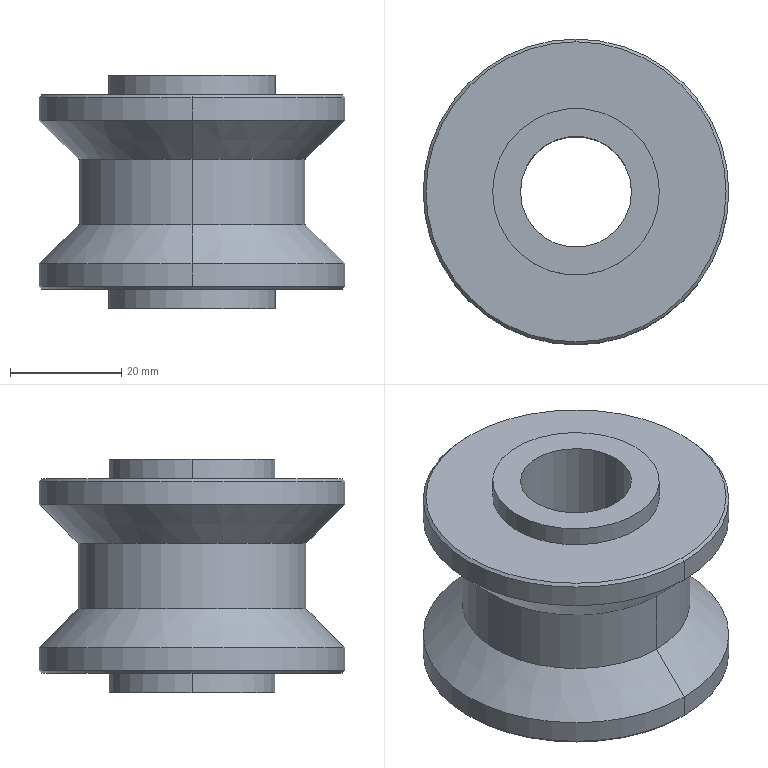Part | NX | features BREP 1 | 1 solid | 24 faces | box 55 x 55 x 42 mm | volume 54660 mm3 | cylinder 12 | cone 8 | plane 4 | commonest cylinder face diameters 30 x4 55 x4 20 x2 41 x2
STEP:
#1=CARTESIAN_POINT('',(-15.,0.,-21.));
#2=VERTEX_POINT('',#1);
#3=CARTESIAN_POINT('',(15.,0.,-21.));
#4=VERTEX_POINT('',#3);
#5=CARTESIAN_POINT('',(0.,0.,-21.));
#6=DIRECTION('',(0.,0.,-1.));
#7=DIRECTION('',(-1.,0.,0.));
#8=AXIS2_PLACEMENT_3D('',#5,#6,#7);
#9=CIRCLE('',#8,15.);
#10=EDGE_CURVE('',#2,#4,#9,.T.);
#11=ORIENTED_EDGE('',*,*,#10,.T.);
#12=CARTESIAN_POINT('',(0.,0.,-21.));
#13=DIRECTION('',(0.,0.,-1.));
#14=DIRECTION('',(1.,0.,0.));
#15=AXIS2_PLACEMENT_3D('',#12,#13,#14);
#16=CIRCLE('',#15,15.);
#17=EDGE_CURVE('',#4,#2,#16,.T.);
#18=ORIENTED_EDGE('',*,*,#17,.T.);
#19=EDGE_LOOP('',(#11,#18));
#20=FACE_BOUND('',#19,.T.);
#21=CARTESIAN_POINT('',(-10.,0.,-21.));
#22=VERTEX_POINT('',#21);
#23=CARTESIAN_POINT('',(10.,0.,-21.));
#24=VERTEX_POINT('',#23);
#25=CARTESIAN_POINT('',(0.,0.,-21.));
#26=DIRECTION('',(0.,0.,1.));
#27=DIRECTION('',(-1.,0.,0.));
#28=AXIS2_PLACEMENT_3D('',#25,#26,#27);
#29=CIRCLE('',#28,10.);
#30=EDGE_CURVE('',#22,#24,#29,.T.);
#31=ORIENTED_EDGE('',*,*,#30,.T.);
#32=CARTESIAN_POINT('',(0.,0.,-21.));
#33=DIRECTION('',(0.,0.,1.));
#34=DIRECTION('',(1.,0.,0.));
#35=AXIS2_PLACEMENT_3D('',#32,#33,#34);
#36=CIRCLE('',#35,10.);
#37=EDGE_CURVE('',#24,#22,#36,.T.);
#38=ORIENTED_EDGE('',*,*,#37,.T.);
#39=EDGE_LOOP('',(#31,#38));
#40=FACE_BOUND('',#39,.T.);
#41=CARTESIAN_POINT('',(0.,0.,-21.));
#42=DIRECTION('',(0.,0.,1.));
#43=DIRECTION('',(1.,0.,0.));
#44=AXIS2_PLACEMENT_3D('',#41,#42,#43);
#45=PLANE('',#44);
#46=ADVANCED_FACE('',(#20,#40),#45,.F.);
#47=ORIENTED_EDGE('',*,*,#17,.F.);
#48=CARTESIAN_POINT('',(15.,0.,-17.5));
#49=VERTEX_POINT('',#48);
#50=CARTESIAN_POINT('',(15.,0.,-17.5));
#51=DIRECTION('',(0.,0.,-1.));
#52=VECTOR('',#51,1000.);
#53=LINE('',#50,#52);
#54=EDGE_CURVE('',#4,#49,#53,.F.);
#55=ORIENTED_EDGE('',*,*,#54,.T.);
#56=CARTESIAN_POINT('',(-15.,0.,-17.5));
#57=VERTEX_POINT('',#56);
#58=CARTESIAN_POINT('',(0.,0.,-17.5));
#59=DIRECTION('',(0.,0.,1.));
#60=DIRECTION('',(-1.,0.,0.));
#61=AXIS2_PLACEMENT_3D('',#58,#59,#60);
#62=CIRCLE('',#61,15.);
#63=EDGE_CURVE('',#57,#49,#62,.T.);
#64=ORIENTED_EDGE('',*,*,#63,.F.);
#65=CARTESIAN_POINT('',(-15.,0.,-17.5));
#66=DIRECTION('',(0.,0.,-1.));
#67=VECTOR('',#66,1000.);
#68=LINE('',#65,#67);
#69=EDGE_CURVE('',#2,#57,#68,.F.);
#70=ORIENTED_EDGE('',*,*,#69,.F.);
#71=EDGE_LOOP('',(#47,#55,#64,#70));
#72=FACE_BOUND('',#71,.T.);
#73=CARTESIAN_POINT('',(0.,0.,0.));
#74=DIRECTION('',(0.,0.,1.));
#75=DIRECTION('',(1.,0.,0.));
#76=AXIS2_PLACEMENT_3D('',#73,#74,#75);
#77=CYLINDRICAL_SURFACE('',#76,15.);
#78=ADVANCED_FACE('',(#72),#77,.T.);
#79=ORIENTED_EDGE('',*,*,#10,.F.);
#80=ORIENTED_EDGE('',*,*,#69,.T.);
#81=CARTESIAN_POINT('',(0.,0.,-17.5));
#82=DIRECTION('',(0.,0.,1.));
#83=DIRECTION('',(1.,0.,0.));
#84=AXIS2_PLACEMENT_3D('',#81,#82,#83);
#85=CIRCLE('',#84,15.);
#86=EDGE_CURVE('',#49,#57,#85,.T.);
#87=ORIENTED_EDGE('',*,*,#86,.F.);
#88=ORIENTED_EDGE('',*,*,#54,.F.);
#89=EDGE_LOOP('',(#79,#80,#87,#88));
#90=FACE_BOUND('',#89,.T.);
#91=CARTESIAN_POINT('',(0.,0.,0.));
#92=DIRECTION('',(0.,0.,1.));
#93=DIRECTION('',(1.,0.,0.));
#94=AXIS2_PLACEMENT_3D('',#91,#92,#93);
#95=CYLINDRICAL_SURFACE('',#94,15.);
#96=ADVANCED_FACE('',(#90),#95,.T.);
#97=CARTESIAN_POINT('',(0.,27.,-17.5));
#98=VERTEX_POINT('',#97);
#99=CARTESIAN_POINT('',(0.,-27.,-17.5));
#100=VERTEX_POINT('',#99);
#101=CARTESIAN_POINT('',(0.,0.,-17.5));
#102=DIRECTION('',(0.,0.,-1.));
#103=DIRECTION('',(0.866,-0.5,0.));
#104=AXIS2_PLACEMENT_3D('',#101,#102,#103);
#105=CIRCLE('',#104,27.);
#106=EDGE_CURVE('',#98,#100,#105,.T.);
#107=ORIENTED_EDGE('',*,*,#106,.T.);
#108=CARTESIAN_POINT('',(0.,0.,-17.5));
#109=DIRECTION('',(0.,0.,-1.));
#110=DIRECTION('',(0.,-1.,0.));
#111=AXIS2_PLACEMENT_3D('',#108,#109,#110);
#112=CIRCLE('',#111,27.);
#113=EDGE_CURVE('',#100,#98,#112,.T.);
#114=ORIENTED_EDGE('',*,*,#113,.T.);
#115=EDGE_LOOP('',(#107,#114));
#116=FACE_BOUND('',#115,.T.);
#117=ORIENTED_EDGE('',*,*,#63,.T.);
#118=ORIENTED_EDGE('',*,*,#86,.T.);
#119=EDGE_LOOP('',(#117,#118));
#120=FACE_BOUND('',#119,.T.);
#121=CARTESIAN_POINT('',(0.,-10.,-17.5));
#122=DIRECTION('',(0.,0.,-1.));
#123=DIRECTION('',(0.,-1.,0.));
#124=AXIS2_PLACEMENT_3D('',#121,#122,#123);
#125=PLANE('',#124);
#126=ADVANCED_FACE('',(#116,#120),#125,.T.);
#127=CARTESIAN_POINT('',(0.,27.5,-17.));
#128=VERTEX_POINT('',#127);
#129=CARTESIAN_POINT('',(0.,-27.5,-17.));
#130=VERTEX_POINT('',#129);
#131=CARTESIAN_POINT('',(0.,0.,-17.));
#132=DIRECTION('',(0.,0.,-1.));
#133=DIRECTION('',(0.,1.,0.));
#134=AXIS2_PLACEMENT_3D('',#131,#132,#133);
#135=CIRCLE('',#134,27.5);
#136=EDGE_CURVE('',#128,#130,#135,.T.);
#137=ORIENTED_EDGE('',*,*,#136,.T.);
#138=CARTESIAN_POINT('',(0.,-27.5,-17.));
#139=DIRECTION('',(0.,0.7071,-0.7071));
#140=VECTOR('',#139,1000.);
#141=LINE('',#138,#140);
#142=EDGE_CURVE('',#130,#100,#141,.T.);
#143=ORIENTED_EDGE('',*,*,#142,.T.);
#144=ORIENTED_EDGE('',*,*,#106,.F.);
#145=CARTESIAN_POINT('',(0.,27.5,-17.));
#146=DIRECTION('',(0.,-0.7071,-0.7071));
#147=VECTOR('',#146,1000.);
#148=LINE('',#145,#147);
#149=EDGE_CURVE('',#128,#98,#148,.T.);
#150=ORIENTED_EDGE('',*,*,#149,.F.);
#151=EDGE_LOOP('',(#137,#143,#144,#150));
#152=FACE_BOUND('',#151,.T.);
#153=CARTESIAN_POINT('',(0.,0.,-17.25));
#154=DIRECTION('',(0.,0.,1.));
#155=DIRECTION('',(-0.866,0.5,0.));
#156=AXIS2_PLACEMENT_3D('',#153,#154,#155);
#157=CONICAL_SURFACE('',#156,27.25,0.7854);
#158=ADVANCED_FACE('',(#152),#157,.T.);
#159=CARTESIAN_POINT('',(0.,0.,-17.));
#160=DIRECTION('',(0.,0.,-1.));
#161=DIRECTION('',(0.,-1.,0.));
#162=AXIS2_PLACEMENT_3D('',#159,#160,#161);
#163=CIRCLE('',#162,27.5);
#164=EDGE_CURVE('',#130,#128,#163,.T.);
#165=ORIENTED_EDGE('',*,*,#164,.T.);
#166=ORIENTED_EDGE('',*,*,#149,.T.);
#167=ORIENTED_EDGE('',*,*,#113,.F.);
#168=ORIENTED_EDGE('',*,*,#142,.F.);
#169=EDGE_LOOP('',(#165,#166,#167,#168));
#170=FACE_BOUND('',#169,.T.);
#171=CARTESIAN_POINT('',(0.,0.,-17.25));
#172=DIRECTION('',(0.,0.,1.));
#173=DIRECTION('',(0.,-1.,0.));
#174=AXIS2_PLACEMENT_3D('',#171,#172,#173);
#175=CONICAL_SURFACE('',#174,27.25,0.7854);
#176=ADVANCED_FACE('',(#170),#175,.T.);
#177=CARTESIAN_POINT('',(0.,27.5,-12.9));
#178=VERTEX_POINT('',#177);
#179=CARTESIAN_POINT('',(0.,-27.5,-12.9));
#180=VERTEX_POINT('',#179);
#181=CARTESIAN_POINT('',(0.,0.,-12.9));
#182=DIRECTION('',(0.,0.,1.));
#183=DIRECTION('',(0.,1.,0.));
#184=AXIS2_PLACEMENT_3D('',#181,#182,#183);
#185=CIRCLE('',#184,27.5);
#186=EDGE_CURVE('',#178,#180,#185,.T.);
#187=ORIENTED_EDGE('',*,*,#186,.F.);
#188=CARTESIAN_POINT('',(0.,27.5,-17.));
#189=DIRECTION('',(0.,0.,1.));
#190=VECTOR('',#189,1000.);
#191=LINE('',#188,#190);
#192=EDGE_CURVE('',#178,#128,#191,.F.);
#193=ORIENTED_EDGE('',*,*,#192,.T.);
#194=ORIENTED_EDGE('',*,*,#164,.F.);
#195=CARTESIAN_POINT('',(0.,-27.5,-17.));
#196=DIRECTION('',(0.,0.,1.));
#197=VECTOR('',#196,1000.);
#198=LINE('',#195,#197);
#199=EDGE_CURVE('',#180,#130,#198,.F.);
#200=ORIENTED_EDGE('',*,*,#199,.F.);
#201=EDGE_LOOP('',(#187,#193,#194,#200));
#202=FACE_BOUND('',#201,.T.);
#203=CARTESIAN_POINT('',(0.,0.,0.));
#204=DIRECTION('',(0.,0.,-1.));
#205=DIRECTION('',(0.,-1.,0.));
#206=AXIS2_PLACEMENT_3D('',#203,#204,#205);
#207=CYLINDRICAL_SURFACE('',#206,27.5);
#208=ADVANCED_FACE('',(#202),#207,.T.);
#209=CARTESIAN_POINT('',(0.,0.,-12.9));
#210=DIRECTION('',(0.,0.,1.));
#211=DIRECTION('',(0.,-1.,0.));
#212=AXIS2_PLACEMENT_3D('',#209,#210,#211);
#213=CIRCLE('',#212,27.5);
#214=EDGE_CURVE('',#180,#178,#213,.T.);
#215=ORIENTED_EDGE('',*,*,#214,.F.);
#216=ORIENTED_EDGE('',*,*,#199,.T.);
#217=ORIENTED_EDGE('',*,*,#136,.F.);
#218=ORIENTED_EDGE('',*,*,#192,.F.);
#219=EDGE_LOOP('',(#215,#216,#217,#218));
#220=FACE_BOUND('',#219,.T.);
#221=CARTESIAN_POINT('',(0.,0.,0.));
#222=DIRECTION('',(0.,0.,-1.));
#223=DIRECTION('',(0.,-1.,0.));
#224=AXIS2_PLACEMENT_3D('',#221,#222,#223);
#225=CYLINDRICAL_SURFACE('',#224,27.5);
#226=ADVANCED_FACE('',(#220),#225,.T.);
#227=ORIENTED_EDGE('',*,*,#214,.T.);
#228=CARTESIAN_POINT('',(0.,20.5,-5.9));
#229=VERTEX_POINT('',#228);
#230=CARTESIAN_POINT('',(0.,27.5,-12.9));
#231=DIRECTION('',(0.,-0.7071,0.7071));
#232=VECTOR('',#231,1000.);
#233=LINE('',#230,#232);
#234=EDGE_CURVE('',#229,#178,#233,.F.);
#235=ORIENTED_EDGE('',*,*,#234,.F.);
#236=CARTESIAN_POINT('',(0.,-20.5,-5.9));
#237=VERTEX_POINT('',#236);
#238=CARTESIAN_POINT('',(0.,0.,-5.9));
#239=DIRECTION('',(0.,0.,-1.));
#240=DIRECTION('',(0.,1.,0.));
#241=AXIS2_PLACEMENT_3D('',#238,#239,#240);
#242=CIRCLE('',#241,20.5);
#243=EDGE_CURVE('',#229,#237,#242,.T.);
#244=ORIENTED_EDGE('',*,*,#243,.T.);
#245=CARTESIAN_POINT('',(0.,-27.5,-12.9));
#246=DIRECTION('',(0.,0.7071,0.7071));
#247=VECTOR('',#246,1000.);
#248=LINE('',#245,#247);
#249=EDGE_CURVE('',#237,#180,#248,.F.);
#250=ORIENTED_EDGE('',*,*,#249,.T.);
#251=EDGE_LOOP('',(#227,#235,#244,#250));
#252=FACE_BOUND('',#251,.T.);
#253=CARTESIAN_POINT('',(0.,0.,-9.4));
#254=DIRECTION('',(0.,0.,-1.));
#255=DIRECTION('',(0.,-1.,0.));
#256=AXIS2_PLACEMENT_3D('',#253,#254,#255);
#257=CONICAL_SURFACE('',#256,24.,0.7854);
#258=ADVANCED_FACE('',(#252),#257,.T.);
#259=ORIENTED_EDGE('',*,*,#186,.T.);
#260=ORIENTED_EDGE('',*,*,#249,.F.);
#261=CARTESIAN_POINT('',(0.,0.,-5.9));
#262=DIRECTION('',(0.,0.,-1.));
#263=DIRECTION('',(0.,-1.,0.));
#264=AXIS2_PLACEMENT_3D('',#261,#262,#263);
#265=CIRCLE('',#264,20.5);
#266=EDGE_CURVE('',#237,#229,#265,.T.);
#267=ORIENTED_EDGE('',*,*,#266,.T.);
#268=ORIENTED_EDGE('',*,*,#234,.T.);
#269=EDGE_LOOP('',(#259,#260,#267,#268));
#270=FACE_BOUND('',#269,.T.);
#271=CARTESIAN_POINT('',(0.,0.,-9.4));
#272=DIRECTION('',(0.,0.,-1.));
#273=DIRECTION('',(0.,-1.,0.));
#274=AXIS2_PLACEMENT_3D('',#271,#272,#273);
#275=CONICAL_SURFACE('',#274,24.,0.7854);
#276=ADVANCED_FACE('',(#270),#275,.T.);
#277=ORIENTED_EDGE('',*,*,#266,.F.);
#278=CARTESIAN_POINT('',(0.,-20.5,5.9));
#279=VERTEX_POINT('',#278);
#280=CARTESIAN_POINT('',(0.,-20.5,-5.9));
#281=DIRECTION('',(0.,0.,1.));
#282=VECTOR('',#281,1000.);
#283=LINE('',#280,#282);
#284=EDGE_CURVE('',#237,#279,#283,.T.);
#285=ORIENTED_EDGE('',*,*,#284,.T.);
#286=CARTESIAN_POINT('',(0.,20.5,5.9));
#287=VERTEX_POINT('',#286);
#288=CARTESIAN_POINT('',(0.,0.,5.9));
#289=DIRECTION('',(0.,0.,1.));
#290=DIRECTION('',(0.,1.,0.));
#291=AXIS2_PLACEMENT_3D('',#288,#289,#290);
#292=CIRCLE('',#291,20.5);
#293=EDGE_CURVE('',#287,#279,#292,.T.);
#294=ORIENTED_EDGE('',*,*,#293,.F.);
#295=CARTESIAN_POINT('',(0.,20.5,-5.9));
#296=DIRECTION('',(0.,0.,1.));
#297=VECTOR('',#296,1000.);
#298=LINE('',#295,#297);
#299=EDGE_CURVE('',#229,#287,#298,.T.);
#300=ORIENTED_EDGE('',*,*,#299,.F.);
#301=EDGE_LOOP('',(#277,#285,#294,#300));
#302=FACE_BOUND('',#301,.T.);
#303=CARTESIAN_POINT('',(0.,0.,0.));
#304=DIRECTION('',(0.,0.,-1.));
#305=DIRECTION('',(0.,-1.,0.));
#306=AXIS2_PLACEMENT_3D('',#303,#304,#305);
#307=CYLINDRICAL_SURFACE('',#306,20.5);
#308=ADVANCED_FACE('',(#302),#307,.T.);
#309=ORIENTED_EDGE('',*,*,#243,.F.);
#310=ORIENTED_EDGE('',*,*,#299,.T.);
#311=CARTESIAN_POINT('',(0.,0.,5.9));
#312=DIRECTION('',(0.,0.,1.));
#313=DIRECTION('',(0.,-1.,0.));
#314=AXIS2_PLACEMENT_3D('',#311,#312,#313);
#315=CIRCLE('',#314,20.5);
#316=EDGE_CURVE('',#279,#287,#315,.T.);
#317=ORIENTED_EDGE('',*,*,#316,.F.);
#318=ORIENTED_EDGE('',*,*,#284,.F.);
#319=EDGE_LOOP('',(#309,#310,#317,#318));
#320=FACE_BOUND('',#319,.T.);
#321=CARTESIAN_POINT('',(0.,0.,0.));
#322=DIRECTION('',(0.,0.,-1.));
#323=DIRECTION('',(0.,-1.,0.));
#324=AXIS2_PLACEMENT_3D('',#321,#322,#323);
#325=CYLINDRICAL_SURFACE('',#324,20.5);
#326=ADVANCED_FACE('',(#320),#325,.T.);
#327=ORIENTED_EDGE('',*,*,#316,.T.);
#328=CARTESIAN_POINT('',(0.,27.5,12.9));
#329=VERTEX_POINT('',#328);
#330=CARTESIAN_POINT('',(0.,20.5,5.9));
#331=DIRECTION('',(0.,0.7071,0.7071));
#332=VECTOR('',#331,1000.);
#333=LINE('',#330,#332);
#334=EDGE_CURVE('',#329,#287,#333,.F.);
#335=ORIENTED_EDGE('',*,*,#334,.F.);
#336=CARTESIAN_POINT('',(0.,-27.5,12.9));
#337=VERTEX_POINT('',#336);
#338=CARTESIAN_POINT('',(0.,0.,12.9));
#339=DIRECTION('',(0.,0.,-1.));
#340=DIRECTION('',(0.,1.,0.));
#341=AXIS2_PLACEMENT_3D('',#338,#339,#340);
#342=CIRCLE('',#341,27.5);
#343=EDGE_CURVE('',#329,#337,#342,.T.);
#344=ORIENTED_EDGE('',*,*,#343,.T.);
#345=CARTESIAN_POINT('',(0.,-20.5,5.9));
#346=DIRECTION('',(0.,-0.7071,0.7071));
#347=VECTOR('',#346,1000.);
#348=LINE('',#345,#347);
#349=EDGE_CURVE('',#337,#279,#348,.F.);
#350=ORIENTED_EDGE('',*,*,#349,.T.);
#351=EDGE_LOOP('',(#327,#335,#344,#350));
#352=FACE_BOUND('',#351,.T.);
#353=CARTESIAN_POINT('',(0.,0.,9.4));
#354=DIRECTION('',(0.,0.,1.));
#355=DIRECTION('',(0.,-1.,0.));
#356=AXIS2_PLACEMENT_3D('',#353,#354,#355);
#357=CONICAL_SURFACE('',#356,24.,0.7854);
#358=ADVANCED_FACE('',(#352),#357,.T.);
#359=ORIENTED_EDGE('',*,*,#293,.T.);
#360=ORIENTED_EDGE('',*,*,#349,.F.);
#361=CARTESIAN_POINT('',(0.,0.,12.9));
#362=DIRECTION('',(0.,0.,-1.));
#363=DIRECTION('',(0.,-1.,0.));
#364=AXIS2_PLACEMENT_3D('',#361,#362,#363);
#365=CIRCLE('',#364,27.5);
#366=EDGE_CURVE('',#337,#329,#365,.T.);
#367=ORIENTED_EDGE('',*,*,#366,.T.);
#368=ORIENTED_EDGE('',*,*,#334,.T.);
#369=EDGE_LOOP('',(#359,#360,#367,#368));
#370=FACE_BOUND('',#369,.T.);
#371=CARTESIAN_POINT('',(0.,0.,9.4));
#372=DIRECTION('',(0.,0.,1.));
#373=DIRECTION('',(0.,-1.,0.));
#374=AXIS2_PLACEMENT_3D('',#371,#372,#373);
#375=CONICAL_SURFACE('',#374,24.,0.7854);
#376=ADVANCED_FACE('',(#370),#375,.T.);
#377=ORIENTED_EDGE('',*,*,#366,.F.);
#378=CARTESIAN_POINT('',(0.,-27.5,17.));
#379=VERTEX_POINT('',#378);
#380=CARTESIAN_POINT('',(0.,-27.5,12.9));
#381=DIRECTION('',(0.,0.,1.));
#382=VECTOR('',#381,1000.);
#383=LINE('',#380,#382);
#384=EDGE_CURVE('',#337,#379,#383,.T.);
#385=ORIENTED_EDGE('',*,*,#384,.T.);
#386=CARTESIAN_POINT('',(0.,27.5,17.));
#387=VERTEX_POINT('',#386);
#388=CARTESIAN_POINT('',(0.,0.,17.));
#389=DIRECTION('',(0.,0.,1.));
#390=DIRECTION('',(0.,1.,0.));
#391=AXIS2_PLACEMENT_3D('',#388,#389,#390);
#392=CIRCLE('',#391,27.5);
#393=EDGE_CURVE('',#387,#379,#392,.T.);
#394=ORIENTED_EDGE('',*,*,#393,.F.);
#395=CARTESIAN_POINT('',(0.,27.5,12.9));
#396=DIRECTION('',(0.,0.,1.));
#397=VECTOR('',#396,1000.);
#398=LINE('',#395,#397);
#399=EDGE_CURVE('',#329,#387,#398,.T.);
#400=ORIENTED_EDGE('',*,*,#399,.F.);
#401=EDGE_LOOP('',(#377,#385,#394,#400));
#402=FACE_BOUND('',#401,.T.);
#403=CARTESIAN_POINT('',(0.,0.,0.));
#404=DIRECTION('',(0.,0.,-1.));
#405=DIRECTION('',(0.,-1.,0.));
#406=AXIS2_PLACEMENT_3D('',#403,#404,#405);
#407=CYLINDRICAL_SURFACE('',#406,27.5);
#408=ADVANCED_FACE('',(#402),#407,.T.);
#409=ORIENTED_EDGE('',*,*,#343,.F.);
#410=ORIENTED_EDGE('',*,*,#399,.T.);
#411=CARTESIAN_POINT('',(0.,0.,17.));
#412=DIRECTION('',(0.,0.,1.));
#413=DIRECTION('',(0.866,-0.5,0.));
#414=AXIS2_PLACEMENT_3D('',#411,#412,#413);
#415=CIRCLE('',#414,27.5);
#416=EDGE_CURVE('',#379,#387,#415,.T.);
#417=ORIENTED_EDGE('',*,*,#416,.F.);
#418=ORIENTED_EDGE('',*,*,#384,.F.);
#419=EDGE_LOOP('',(#409,#410,#417,#418));
#420=FACE_BOUND('',#419,.T.);
#421=CARTESIAN_POINT('',(0.,0.,0.));
#422=DIRECTION('',(0.,0.,-1.));
#423=DIRECTION('',(0.,-1.,0.));
#424=AXIS2_PLACEMENT_3D('',#421,#422,#423);
#425=CYLINDRICAL_SURFACE('',#424,27.5);
#426=ADVANCED_FACE('',(#420),#425,.T.);
#427=CARTESIAN_POINT('',(0.,-27.,17.5));
#428=VERTEX_POINT('',#427);
#429=CARTESIAN_POINT('',(0.,27.,17.5));
#430=VERTEX_POINT('',#429);
#431=CARTESIAN_POINT('',(0.,0.,17.5));
#432=DIRECTION('',(0.,0.,1.));
#433=DIRECTION('',(0.866,-0.5,0.));
#434=AXIS2_PLACEMENT_3D('',#431,#432,#433);
#435=CIRCLE('',#434,27.);
#436=EDGE_CURVE('',#428,#430,#435,.T.);
#437=ORIENTED_EDGE('',*,*,#436,.F.);
#438=CARTESIAN_POINT('',(0.,-27.,17.5));
#439=DIRECTION('',(0.,-0.7071,-0.7071));
#440=VECTOR('',#439,1000.);
#441=LINE('',#438,#440);
#442=EDGE_CURVE('',#428,#379,#441,.T.);
#443=ORIENTED_EDGE('',*,*,#442,.T.);
#444=ORIENTED_EDGE('',*,*,#416,.T.);
#445=CARTESIAN_POINT('',(0.,27.,17.5));
#446=DIRECTION('',(0.,0.7071,-0.7071));
#447=VECTOR('',#446,1000.);
#448=LINE('',#445,#447);
#449=EDGE_CURVE('',#430,#387,#448,.T.);
#450=ORIENTED_EDGE('',*,*,#449,.F.);
#451=EDGE_LOOP('',(#437,#443,#444,#450));
#452=FACE_BOUND('',#451,.T.);
#453=CARTESIAN_POINT('',(0.,0.,17.25));
#454=DIRECTION('',(0.,0.,-1.));
#455=DIRECTION('',(-0.866,0.5,0.));
#456=AXIS2_PLACEMENT_3D('',#453,#454,#455);
#457=CONICAL_SURFACE('',#456,27.25,0.7854);
#458=ADVANCED_FACE('',(#452),#457,.T.);
#459=CARTESIAN_POINT('',(0.,0.,17.5));
#460=DIRECTION('',(0.,0.,1.));
#461=DIRECTION('',(0.,1.,0.));
#462=AXIS2_PLACEMENT_3D('',#459,#460,#461);
#463=CIRCLE('',#462,27.);
#464=EDGE_CURVE('',#430,#428,#463,.T.);
#465=ORIENTED_EDGE('',*,*,#464,.F.);
#466=ORIENTED_EDGE('',*,*,#449,.T.);
#467=ORIENTED_EDGE('',*,*,#393,.T.);
#468=ORIENTED_EDGE('',*,*,#442,.F.);
#469=EDGE_LOOP('',(#465,#466,#467,#468));
#470=FACE_BOUND('',#469,.T.);
#471=CARTESIAN_POINT('',(0.,0.,17.25));
#472=DIRECTION('',(0.,0.,-1.));
#473=DIRECTION('',(0.,-1.,0.));
#474=AXIS2_PLACEMENT_3D('',#471,#472,#473);
#475=CONICAL_SURFACE('',#474,27.25,0.7854);
#476=ADVANCED_FACE('',(#470),#475,.T.);
#477=ORIENTED_EDGE('',*,*,#464,.T.);
#478=ORIENTED_EDGE('',*,*,#436,.T.);
#479=EDGE_LOOP('',(#477,#478));
#480=FACE_BOUND('',#479,.T.);
#481=CARTESIAN_POINT('',(-15.,0.,17.5));
#482=VERTEX_POINT('',#481);
#483=CARTESIAN_POINT('',(15.,0.,17.5));
#484=VERTEX_POINT('',#483);
#485=CARTESIAN_POINT('',(0.,0.,17.5));
#486=DIRECTION('',(0.,0.,-1.));
#487=DIRECTION('',(-1.,0.,0.));
#488=AXIS2_PLACEMENT_3D('',#485,#486,#487);
#489=CIRCLE('',#488,15.);
#490=EDGE_CURVE('',#482,#484,#489,.T.);
#491=ORIENTED_EDGE('',*,*,#490,.T.);
#492=CARTESIAN_POINT('',(0.,0.,17.5));
#493=DIRECTION('',(0.,0.,-1.));
#494=DIRECTION('',(1.,0.,0.));
#495=AXIS2_PLACEMENT_3D('',#492,#493,#494);
#496=CIRCLE('',#495,15.);
#497=EDGE_CURVE('',#484,#482,#496,.T.);
#498=ORIENTED_EDGE('',*,*,#497,.T.);
#499=EDGE_LOOP('',(#491,#498));
#500=FACE_BOUND('',#499,.T.);
#501=CARTESIAN_POINT('',(0.,-27.5,17.5));
#502=DIRECTION('',(0.,0.,-1.));
#503=DIRECTION('',(0.,-1.,0.));
#504=AXIS2_PLACEMENT_3D('',#501,#502,#503);
#505=PLANE('',#504);
#506=ADVANCED_FACE('',(#480,#500),#505,.F.);
#507=CARTESIAN_POINT('',(-15.,0.,21.));
#508=VERTEX_POINT('',#507);
#509=CARTESIAN_POINT('',(15.,0.,21.));
#510=VERTEX_POINT('',#509);
#511=CARTESIAN_POINT('',(0.,0.,21.));
#512=DIRECTION('',(0.,0.,1.));
#513=DIRECTION('',(-1.,0.,0.));
#514=AXIS2_PLACEMENT_3D('',#511,#512,#513);
#515=CIRCLE('',#514,15.);
#516=EDGE_CURVE('',#508,#510,#515,.T.);
#517=ORIENTED_EDGE('',*,*,#516,.F.);
#518=CARTESIAN_POINT('',(-15.,0.,21.));
#519=DIRECTION('',(0.,0.,-1.));
#520=VECTOR('',#519,1000.);
#521=LINE('',#518,#520);
#522=EDGE_CURVE('',#508,#482,#521,.T.);
#523=ORIENTED_EDGE('',*,*,#522,.T.);
#524=ORIENTED_EDGE('',*,*,#497,.F.);
#525=CARTESIAN_POINT('',(15.,0.,21.));
#526=DIRECTION('',(0.,0.,-1.));
#527=VECTOR('',#526,1000.);
#528=LINE('',#525,#527);
#529=EDGE_CURVE('',#510,#484,#528,.T.);
#530=ORIENTED_EDGE('',*,*,#529,.F.);
#531=EDGE_LOOP('',(#517,#523,#524,#530));
#532=FACE_BOUND('',#531,.T.);
#533=CARTESIAN_POINT('',(0.,0.,0.));
#534=DIRECTION('',(0.,0.,1.));
#535=DIRECTION('',(1.,0.,0.));
#536=AXIS2_PLACEMENT_3D('',#533,#534,#535);
#537=CYLINDRICAL_SURFACE('',#536,15.);
#538=ADVANCED_FACE('',(#532),#537,.T.);
#539=CARTESIAN_POINT('',(0.,0.,21.));
#540=DIRECTION('',(0.,0.,1.));
#541=DIRECTION('',(1.,0.,0.));
#542=AXIS2_PLACEMENT_3D('',#539,#540,#541);
#543=CIRCLE('',#542,15.);
#544=EDGE_CURVE('',#510,#508,#543,.T.);
#545=ORIENTED_EDGE('',*,*,#544,.F.);
#546=ORIENTED_EDGE('',*,*,#529,.T.);
#547=ORIENTED_EDGE('',*,*,#490,.F.);
#548=ORIENTED_EDGE('',*,*,#522,.F.);
#549=EDGE_LOOP('',(#545,#546,#547,#548));
#550=FACE_BOUND('',#549,.T.);
#551=CARTESIAN_POINT('',(0.,0.,0.));
#552=DIRECTION('',(0.,0.,1.));
#553=DIRECTION('',(1.,0.,0.));
#554=AXIS2_PLACEMENT_3D('',#551,#552,#553);
#555=CYLINDRICAL_SURFACE('',#554,15.);
#556=ADVANCED_FACE('',(#550),#555,.T.);
#557=ORIENTED_EDGE('',*,*,#516,.T.);
#558=ORIENTED_EDGE('',*,*,#544,.T.);
#559=EDGE_LOOP('',(#557,#558));
#560=FACE_BOUND('',#559,.T.);
#561=CARTESIAN_POINT('',(-10.,0.,21.));
#562=VERTEX_POINT('',#561);
#563=CARTESIAN_POINT('',(10.,0.,21.));
#564=VERTEX_POINT('',#563);
#565=CARTESIAN_POINT('',(0.,0.,21.));
#566=DIRECTION('',(0.,0.,-1.));
#567=DIRECTION('',(-1.,0.,0.));
#568=AXIS2_PLACEMENT_3D('',#565,#566,#567);
#569=CIRCLE('',#568,10.);
#570=EDGE_CURVE('',#562,#564,#569,.T.);
#571=ORIENTED_EDGE('',*,*,#570,.T.);
#572=CARTESIAN_POINT('',(0.,0.,21.));
#573=DIRECTION('',(0.,0.,-1.));
#574=DIRECTION('',(1.,0.,0.));
#575=AXIS2_PLACEMENT_3D('',#572,#573,#574);
#576=CIRCLE('',#575,10.);
#577=EDGE_CURVE('',#564,#562,#576,.T.);
#578=ORIENTED_EDGE('',*,*,#577,.T.);
#579=EDGE_LOOP('',(#571,#578));
#580=FACE_BOUND('',#579,.T.);
#581=CARTESIAN_POINT('',(0.,0.,21.));
#582=DIRECTION('',(0.,0.,1.));
#583=DIRECTION('',(1.,0.,0.));
#584=AXIS2_PLACEMENT_3D('',#581,#582,#583);
#585=PLANE('',#584);
#586=ADVANCED_FACE('',(#560,#580),#585,.T.);
#587=CARTESIAN_POINT('',(-10.,0.,21.));
#588=DIRECTION('',(0.,0.,-1.));
#589=VECTOR('',#588,1000.);
#590=LINE('',#587,#589);
#591=EDGE_CURVE('',#22,#562,#590,.F.);
#592=ORIENTED_EDGE('',*,*,#591,.T.);
#593=ORIENTED_EDGE('',*,*,#577,.F.);
#594=CARTESIAN_POINT('',(10.,0.,21.));
#595=DIRECTION('',(0.,0.,-1.));
#596=VECTOR('',#595,1000.);
#597=LINE('',#594,#596);
#598=EDGE_CURVE('',#24,#564,#597,.F.);
#599=ORIENTED_EDGE('',*,*,#598,.F.);
#600=ORIENTED_EDGE('',*,*,#30,.F.);
#601=EDGE_LOOP('',(#592,#593,#599,#600));
#602=FACE_BOUND('',#601,.T.);
#603=CARTESIAN_POINT('',(0.,0.,0.));
#604=DIRECTION('',(0.,0.,1.));
#605=DIRECTION('',(1.,0.,0.));
#606=AXIS2_PLACEMENT_3D('',#603,#604,#605);
#607=CYLINDRICAL_SURFACE('',#606,10.);
#608=ADVANCED_FACE('',(#602),#607,.F.);
#609=ORIENTED_EDGE('',*,*,#591,.F.);
#610=ORIENTED_EDGE('',*,*,#37,.F.);
#611=ORIENTED_EDGE('',*,*,#598,.T.);
#612=ORIENTED_EDGE('',*,*,#570,.F.);
#613=EDGE_LOOP('',(#609,#610,#611,#612));
#614=FACE_BOUND('',#613,.T.);
#615=CARTESIAN_POINT('',(0.,0.,0.));
#616=DIRECTION('',(0.,0.,1.));
#617=DIRECTION('',(1.,0.,0.));
#618=AXIS2_PLACEMENT_3D('',#615,#616,#617);
#619=CYLINDRICAL_SURFACE('',#618,10.);
#620=ADVANCED_FACE('',(#614),#619,.F.);
#621=CLOSED_SHELL('',(#46,#78,#96,#126,#158,#176,#208,#226,#258,#276,#308,#326,#358,#376,#408,#426,#458,#476,#506,#538,#556,#586,#608,#620));
#622=MANIFOLD_SOLID_BREP('',#621);
#623=(LENGTH_UNIT()NAMED_UNIT(*)SI_UNIT(.MILLI.,.METRE.));
#624=UNCERTAINTY_MEASURE_WITH_UNIT(LENGTH_MEASURE(0.00001),#623,'','');
#625=(NAMED_UNIT(*)PLANE_ANGLE_UNIT()SI_UNIT($,.RADIAN.));
#626=(NAMED_UNIT(*)SI_UNIT($,.STERADIAN.)SOLID_ANGLE_UNIT());
#627=(GEOMETRIC_REPRESENTATION_CONTEXT(3)GLOBAL_UNCERTAINTY_ASSIGNED_CONTEXT((#624))GLOBAL_UNIT_ASSIGNED_CONTEXT((#623,#625,#626))REPRESENTATION_CONTEXT('',''));
#628=ADVANCED_BREP_SHAPE_REPRESENTATION('',(#622),#627);